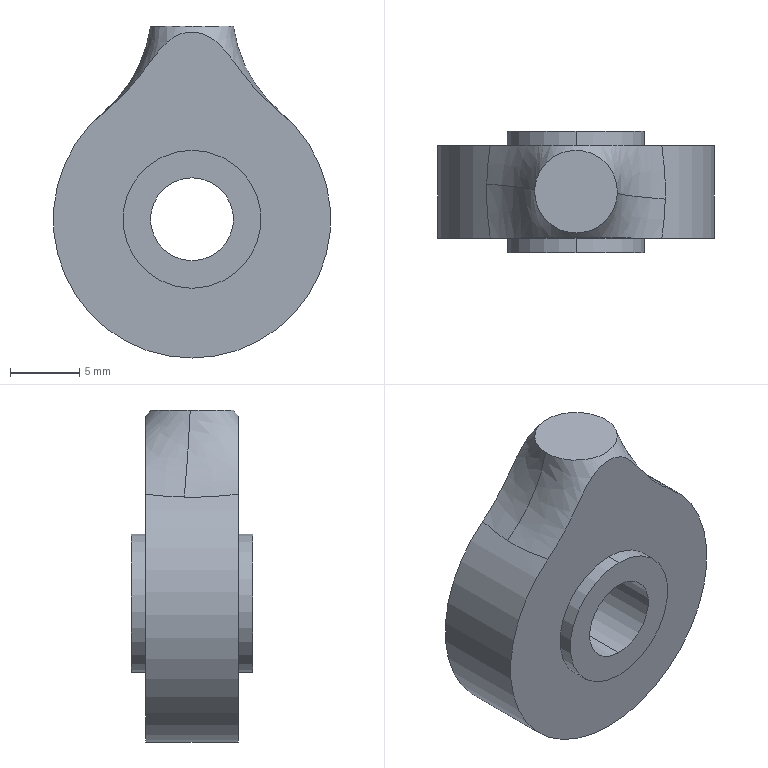Part | SolidWorks | features ICE 3, Extrusion 1, Fillet 1 | 1 solid | 15 faces | volume 2238 mm3 | cylinder 8 | plane 5 | spline 2 | commonest cylinder face diameters 10 x4 6 x2 20.1 x2